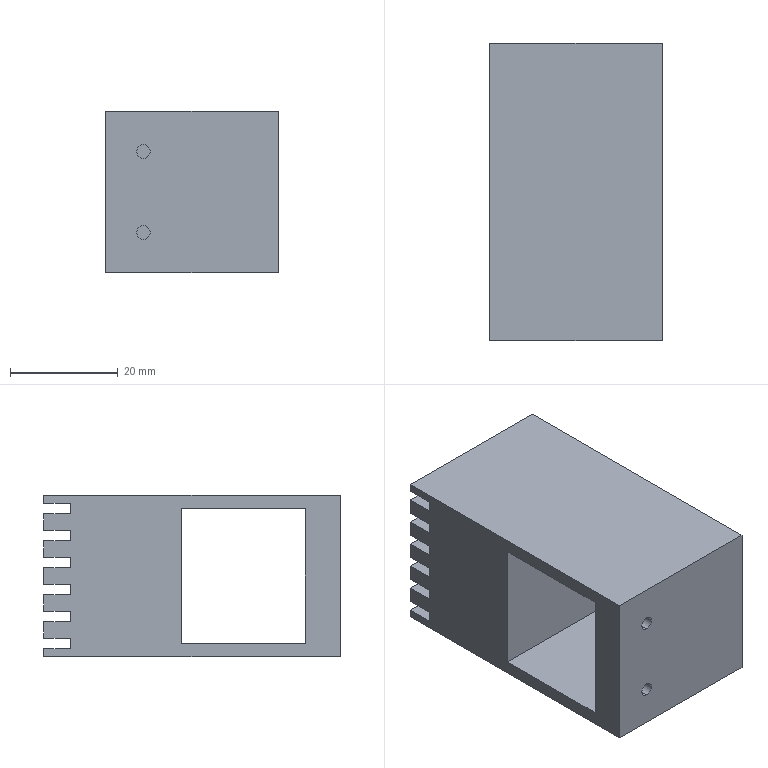Part | SolidWorks | features ICE 2, Extrusion 1, HoleWzd 1, LPattern 1 | 1 solid | 38 faces | box 32 x 55 x 30 mm | volume 32416 mm3 | plane 34 | cylinder 4 | commonest cylinder face diameters 2.5 x4
STEP:
#1=CARTESIAN_POINT('',(-9.,6.5,-8.75));
#2=VERTEX_POINT('',#1);
#3=CARTESIAN_POINT('',(-9.,6.5,-6.25));
#4=VERTEX_POINT('',#3);
#5=CARTESIAN_POINT('',(-9.,6.5,-7.5));
#6=DIRECTION('',(0.,1.,0.));
#7=DIRECTION('',(0.,0.,-1.));
#8=AXIS2_PLACEMENT_3D('',#5,#6,#7);
#9=CIRCLE('',#8,1.25);
#10=EDGE_CURVE('',#2,#4,#9,.T.);
#11=ORIENTED_EDGE('',*,*,#10,.T.);
#12=CARTESIAN_POINT('',(-9.,0.,-6.25));
#13=VERTEX_POINT('',#12);
#14=CARTESIAN_POINT('',(-9.,0.,-6.25));
#15=DIRECTION('',(0.,-1.,0.));
#16=VECTOR('',#15,1000.);
#17=LINE('',#14,#16);
#18=EDGE_CURVE('',#4,#13,#17,.T.);
#19=ORIENTED_EDGE('',*,*,#18,.T.);
#20=CARTESIAN_POINT('',(-9.,0.,-8.75));
#21=VERTEX_POINT('',#20);
#22=CARTESIAN_POINT('',(-9.,0.,-7.5));
#23=DIRECTION('',(0.,-1.,0.));
#24=DIRECTION('',(0.,0.,-1.));
#25=AXIS2_PLACEMENT_3D('',#22,#23,#24);
#26=CIRCLE('',#25,1.25);
#27=EDGE_CURVE('',#13,#21,#26,.T.);
#28=ORIENTED_EDGE('',*,*,#27,.T.);
#29=CARTESIAN_POINT('',(-9.,0.,-8.75));
#30=DIRECTION('',(0.,-1.,0.));
#31=VECTOR('',#30,1000.);
#32=LINE('',#29,#31);
#33=EDGE_CURVE('',#2,#21,#32,.T.);
#34=ORIENTED_EDGE('',*,*,#33,.F.);
#35=EDGE_LOOP('',(#11,#19,#28,#34));
#36=FACE_OUTER_BOUND('',#35,.T.);
#37=CARTESIAN_POINT('',(-9.,0.,-7.5));
#38=DIRECTION('',(0.,-1.,0.));
#39=DIRECTION('',(0.,0.,-1.));
#40=AXIS2_PLACEMENT_3D('',#37,#38,#39);
#41=CYLINDRICAL_SURFACE('',#40,1.25);
#42=ADVANCED_FACE('',(#36),#41,.F.);
#43=CARTESIAN_POINT('',(-9.,6.5,6.25));
#44=VERTEX_POINT('',#43);
#45=CARTESIAN_POINT('',(-9.,6.5,8.75));
#46=VERTEX_POINT('',#45);
#47=CARTESIAN_POINT('',(-9.,6.5,7.5));
#48=DIRECTION('',(0.,1.,0.));
#49=DIRECTION('',(0.,0.,-1.));
#50=AXIS2_PLACEMENT_3D('',#47,#48,#49);
#51=CIRCLE('',#50,1.25);
#52=EDGE_CURVE('',#44,#46,#51,.T.);
#53=ORIENTED_EDGE('',*,*,#52,.T.);
#54=CARTESIAN_POINT('',(-9.,0.,8.75));
#55=VERTEX_POINT('',#54);
#56=CARTESIAN_POINT('',(-9.,0.,8.75));
#57=DIRECTION('',(0.,-1.,0.));
#58=VECTOR('',#57,1000.);
#59=LINE('',#56,#58);
#60=EDGE_CURVE('',#46,#55,#59,.T.);
#61=ORIENTED_EDGE('',*,*,#60,.T.);
#62=CARTESIAN_POINT('',(-9.,0.,6.25));
#63=VERTEX_POINT('',#62);
#64=CARTESIAN_POINT('',(-9.,0.,7.5));
#65=DIRECTION('',(0.,-1.,0.));
#66=DIRECTION('',(0.,0.,-1.));
#67=AXIS2_PLACEMENT_3D('',#64,#65,#66);
#68=CIRCLE('',#67,1.25);
#69=EDGE_CURVE('',#55,#63,#68,.T.);
#70=ORIENTED_EDGE('',*,*,#69,.T.);
#71=CARTESIAN_POINT('',(-9.,0.,6.25));
#72=DIRECTION('',(0.,-1.,0.));
#73=VECTOR('',#72,1000.);
#74=LINE('',#71,#73);
#75=EDGE_CURVE('',#44,#63,#74,.T.);
#76=ORIENTED_EDGE('',*,*,#75,.F.);
#77=EDGE_LOOP('',(#53,#61,#70,#76));
#78=FACE_OUTER_BOUND('',#77,.T.);
#79=CARTESIAN_POINT('',(-9.,0.,7.5));
#80=DIRECTION('',(0.,-1.,0.));
#81=DIRECTION('',(0.,0.,-1.));
#82=AXIS2_PLACEMENT_3D('',#79,#80,#81);
#83=CYLINDRICAL_SURFACE('',#82,1.25);
#84=ADVANCED_FACE('',(#78),#83,.F.);
#85=CARTESIAN_POINT('',(-16.,55.,8.5));
#86=VERTEX_POINT('',#85);
#87=CARTESIAN_POINT('',(16.,55.,8.5));
#88=VERTEX_POINT('',#87);
#89=CARTESIAN_POINT('',(-16.,55.,8.5));
#90=DIRECTION('',(1.,0.,0.));
#91=VECTOR('',#90,1000.);
#92=LINE('',#89,#91);
#93=EDGE_CURVE('',#86,#88,#92,.T.);
#94=ORIENTED_EDGE('',*,*,#93,.F.);
#95=CARTESIAN_POINT('',(-16.,55.,11.5));
#96=VERTEX_POINT('',#95);
#97=CARTESIAN_POINT('',(-16.,55.,-15.));
#98=DIRECTION('',(0.,0.,1.));
#99=VECTOR('',#98,1000.);
#100=LINE('',#97,#99);
#101=EDGE_CURVE('',#86,#96,#100,.T.);
#102=ORIENTED_EDGE('',*,*,#101,.T.);
#103=CARTESIAN_POINT('',(16.,55.,11.5));
#104=VERTEX_POINT('',#103);
#105=CARTESIAN_POINT('',(-16.,55.,11.5));
#106=DIRECTION('',(1.,0.,0.));
#107=VECTOR('',#106,1000.);
#108=LINE('',#105,#107);
#109=EDGE_CURVE('',#96,#104,#108,.T.);
#110=ORIENTED_EDGE('',*,*,#109,.T.);
#111=CARTESIAN_POINT('',(16.,55.,-15.));
#112=DIRECTION('',(0.,0.,-1.));
#113=VECTOR('',#112,1000.);
#114=LINE('',#111,#113);
#115=EDGE_CURVE('',#104,#88,#114,.T.);
#116=ORIENTED_EDGE('',*,*,#115,.T.);
#117=EDGE_LOOP('',(#94,#102,#110,#116));
#118=FACE_OUTER_BOUND('',#117,.T.);
#119=CARTESIAN_POINT('',(0.,55.,0.));
#120=DIRECTION('',(0.,1.,0.));
#121=DIRECTION('',(0.,0.,1.));
#122=AXIS2_PLACEMENT_3D('',#119,#120,#121);
#123=PLANE('',#122);
#124=ADVANCED_FACE('',(#118),#123,.T.);
#125=CARTESIAN_POINT('',(-16.,55.,6.5));
#126=VERTEX_POINT('',#125);
#127=CARTESIAN_POINT('',(16.,55.,6.5));
#128=VERTEX_POINT('',#127);
#129=CARTESIAN_POINT('',(-16.,55.,6.5));
#130=DIRECTION('',(1.,0.,0.));
#131=VECTOR('',#130,1000.);
#132=LINE('',#129,#131);
#133=EDGE_CURVE('',#126,#128,#132,.T.);
#134=ORIENTED_EDGE('',*,*,#133,.T.);
#135=CARTESIAN_POINT('',(16.,55.,3.5));
#136=VERTEX_POINT('',#135);
#137=CARTESIAN_POINT('',(16.,55.,-15.));
#138=DIRECTION('',(0.,0.,-1.));
#139=VECTOR('',#138,1000.);
#140=LINE('',#137,#139);
#141=EDGE_CURVE('',#128,#136,#140,.T.);
#142=ORIENTED_EDGE('',*,*,#141,.T.);
#143=CARTESIAN_POINT('',(-16.,55.,3.5));
#144=VERTEX_POINT('',#143);
#145=CARTESIAN_POINT('',(-16.,55.,3.5));
#146=DIRECTION('',(1.,0.,0.));
#147=VECTOR('',#146,1000.);
#148=LINE('',#145,#147);
#149=EDGE_CURVE('',#144,#136,#148,.T.);
#150=ORIENTED_EDGE('',*,*,#149,.F.);
#151=CARTESIAN_POINT('',(-16.,55.,-15.));
#152=DIRECTION('',(0.,0.,1.));
#153=VECTOR('',#152,1000.);
#154=LINE('',#151,#153);
#155=EDGE_CURVE('',#144,#126,#154,.T.);
#156=ORIENTED_EDGE('',*,*,#155,.T.);
#157=EDGE_LOOP('',(#134,#142,#150,#156));
#158=FACE_OUTER_BOUND('',#157,.T.);
#159=CARTESIAN_POINT('',(0.,55.,0.));
#160=DIRECTION('',(0.,1.,0.));
#161=DIRECTION('',(0.,0.,1.));
#162=AXIS2_PLACEMENT_3D('',#159,#160,#161);
#163=PLANE('',#162);
#164=ADVANCED_FACE('',(#158),#163,.T.);
#165=CARTESIAN_POINT('',(-16.,55.,1.5));
#166=VERTEX_POINT('',#165);
#167=CARTESIAN_POINT('',(16.,55.,1.5));
#168=VERTEX_POINT('',#167);
#169=CARTESIAN_POINT('',(-16.,55.,1.5));
#170=DIRECTION('',(1.,0.,0.));
#171=VECTOR('',#170,1000.);
#172=LINE('',#169,#171);
#173=EDGE_CURVE('',#166,#168,#172,.T.);
#174=ORIENTED_EDGE('',*,*,#173,.T.);
#175=CARTESIAN_POINT('',(16.,55.,-1.5));
#176=VERTEX_POINT('',#175);
#177=CARTESIAN_POINT('',(16.,55.,-15.));
#178=DIRECTION('',(0.,0.,-1.));
#179=VECTOR('',#178,1000.);
#180=LINE('',#177,#179);
#181=EDGE_CURVE('',#168,#176,#180,.T.);
#182=ORIENTED_EDGE('',*,*,#181,.T.);
#183=CARTESIAN_POINT('',(-16.,55.,-1.5));
#184=VERTEX_POINT('',#183);
#185=CARTESIAN_POINT('',(-16.,55.,-1.5));
#186=DIRECTION('',(1.,0.,0.));
#187=VECTOR('',#186,1000.);
#188=LINE('',#185,#187);
#189=EDGE_CURVE('',#184,#176,#188,.T.);
#190=ORIENTED_EDGE('',*,*,#189,.F.);
#191=CARTESIAN_POINT('',(-16.,55.,-15.));
#192=DIRECTION('',(0.,0.,1.));
#193=VECTOR('',#192,1000.);
#194=LINE('',#191,#193);
#195=EDGE_CURVE('',#184,#166,#194,.T.);
#196=ORIENTED_EDGE('',*,*,#195,.T.);
#197=EDGE_LOOP('',(#174,#182,#190,#196));
#198=FACE_OUTER_BOUND('',#197,.T.);
#199=CARTESIAN_POINT('',(0.,55.,0.));
#200=DIRECTION('',(0.,1.,0.));
#201=DIRECTION('',(0.,0.,1.));
#202=AXIS2_PLACEMENT_3D('',#199,#200,#201);
#203=PLANE('',#202);
#204=ADVANCED_FACE('',(#198),#203,.T.);
#205=CARTESIAN_POINT('',(-16.,55.,-3.5));
#206=VERTEX_POINT('',#205);
#207=CARTESIAN_POINT('',(16.,55.,-3.5));
#208=VERTEX_POINT('',#207);
#209=CARTESIAN_POINT('',(-16.,55.,-3.5));
#210=DIRECTION('',(1.,0.,0.));
#211=VECTOR('',#210,1000.);
#212=LINE('',#209,#211);
#213=EDGE_CURVE('',#206,#208,#212,.T.);
#214=ORIENTED_EDGE('',*,*,#213,.T.);
#215=CARTESIAN_POINT('',(16.,55.,-6.5));
#216=VERTEX_POINT('',#215);
#217=CARTESIAN_POINT('',(16.,55.,-15.));
#218=DIRECTION('',(0.,0.,-1.));
#219=VECTOR('',#218,1000.);
#220=LINE('',#217,#219);
#221=EDGE_CURVE('',#208,#216,#220,.T.);
#222=ORIENTED_EDGE('',*,*,#221,.T.);
#223=CARTESIAN_POINT('',(-16.,55.,-6.5));
#224=VERTEX_POINT('',#223);
#225=CARTESIAN_POINT('',(-16.,55.,-6.5));
#226=DIRECTION('',(1.,0.,0.));
#227=VECTOR('',#226,1000.);
#228=LINE('',#225,#227);
#229=EDGE_CURVE('',#224,#216,#228,.T.);
#230=ORIENTED_EDGE('',*,*,#229,.F.);
#231=CARTESIAN_POINT('',(-16.,55.,-15.));
#232=DIRECTION('',(0.,0.,1.));
#233=VECTOR('',#232,1000.);
#234=LINE('',#231,#233);
#235=EDGE_CURVE('',#224,#206,#234,.T.);
#236=ORIENTED_EDGE('',*,*,#235,.T.);
#237=EDGE_LOOP('',(#214,#222,#230,#236));
#238=FACE_OUTER_BOUND('',#237,.T.);
#239=CARTESIAN_POINT('',(0.,55.,0.));
#240=DIRECTION('',(0.,1.,0.));
#241=DIRECTION('',(0.,0.,1.));
#242=AXIS2_PLACEMENT_3D('',#239,#240,#241);
#243=PLANE('',#242);
#244=ADVANCED_FACE('',(#238),#243,.T.);
#245=CARTESIAN_POINT('',(-16.,55.,-8.5));
#246=VERTEX_POINT('',#245);
#247=CARTESIAN_POINT('',(16.,55.,-8.5));
#248=VERTEX_POINT('',#247);
#249=CARTESIAN_POINT('',(-16.,55.,-8.5));
#250=DIRECTION('',(1.,0.,0.));
#251=VECTOR('',#250,1000.);
#252=LINE('',#249,#251);
#253=EDGE_CURVE('',#246,#248,#252,.T.);
#254=ORIENTED_EDGE('',*,*,#253,.T.);
#255=CARTESIAN_POINT('',(16.,55.,-11.5));
#256=VERTEX_POINT('',#255);
#257=CARTESIAN_POINT('',(16.,55.,-15.));
#258=DIRECTION('',(0.,0.,-1.));
#259=VECTOR('',#258,1000.);
#260=LINE('',#257,#259);
#261=EDGE_CURVE('',#248,#256,#260,.T.);
#262=ORIENTED_EDGE('',*,*,#261,.T.);
#263=CARTESIAN_POINT('',(-16.,55.,-11.5));
#264=VERTEX_POINT('',#263);
#265=CARTESIAN_POINT('',(-16.,55.,-11.5));
#266=DIRECTION('',(1.,0.,0.));
#267=VECTOR('',#266,1000.);
#268=LINE('',#265,#267);
#269=EDGE_CURVE('',#264,#256,#268,.T.);
#270=ORIENTED_EDGE('',*,*,#269,.F.);
#271=CARTESIAN_POINT('',(-16.,55.,-15.));
#272=DIRECTION('',(0.,0.,1.));
#273=VECTOR('',#272,1000.);
#274=LINE('',#271,#273);
#275=EDGE_CURVE('',#264,#246,#274,.T.);
#276=ORIENTED_EDGE('',*,*,#275,.T.);
#277=EDGE_LOOP('',(#254,#262,#270,#276));
#278=FACE_OUTER_BOUND('',#277,.T.);
#279=CARTESIAN_POINT('',(0.,55.,0.));
#280=DIRECTION('',(0.,1.,0.));
#281=DIRECTION('',(0.,0.,1.));
#282=AXIS2_PLACEMENT_3D('',#279,#280,#281);
#283=PLANE('',#282);
#284=ADVANCED_FACE('',(#278),#283,.T.);
#285=CARTESIAN_POINT('',(-16.,55.,13.5));
#286=VERTEX_POINT('',#285);
#287=CARTESIAN_POINT('',(16.,55.,13.5));
#288=VERTEX_POINT('',#287);
#289=CARTESIAN_POINT('',(-16.,55.,13.5));
#290=DIRECTION('',(1.,0.,0.));
#291=VECTOR('',#290,1000.);
#292=LINE('',#289,#291);
#293=EDGE_CURVE('',#286,#288,#292,.T.);
#294=ORIENTED_EDGE('',*,*,#293,.F.);
#295=CARTESIAN_POINT('',(-16.,55.,15.));
#296=VERTEX_POINT('',#295);
#297=CARTESIAN_POINT('',(-16.,55.,-15.));
#298=DIRECTION('',(0.,0.,1.));
#299=VECTOR('',#298,1000.);
#300=LINE('',#297,#299);
#301=EDGE_CURVE('',#286,#296,#300,.T.);
#302=ORIENTED_EDGE('',*,*,#301,.T.);
#303=CARTESIAN_POINT('',(16.,55.,15.));
#304=VERTEX_POINT('',#303);
#305=CARTESIAN_POINT('',(-16.,55.,15.));
#306=DIRECTION('',(1.,0.,0.));
#307=VECTOR('',#306,1000.);
#308=LINE('',#305,#307);
#309=EDGE_CURVE('',#296,#304,#308,.T.);
#310=ORIENTED_EDGE('',*,*,#309,.T.);
#311=CARTESIAN_POINT('',(16.,55.,-15.));
#312=DIRECTION('',(0.,0.,-1.));
#313=VECTOR('',#312,1000.);
#314=LINE('',#311,#313);
#315=EDGE_CURVE('',#304,#288,#314,.T.);
#316=ORIENTED_EDGE('',*,*,#315,.T.);
#317=EDGE_LOOP('',(#294,#302,#310,#316));
#318=FACE_OUTER_BOUND('',#317,.T.);
#319=CARTESIAN_POINT('',(0.,55.,0.));
#320=DIRECTION('',(0.,1.,0.));
#321=DIRECTION('',(0.,0.,1.));
#322=AXIS2_PLACEMENT_3D('',#319,#320,#321);
#323=PLANE('',#322);
#324=ADVANCED_FACE('',(#318),#323,.T.);
#325=CARTESIAN_POINT('',(16.,6.5,12.5));
#326=VERTEX_POINT('',#325);
#327=CARTESIAN_POINT('',(16.,6.5,-12.5));
#328=VERTEX_POINT('',#327);
#329=CARTESIAN_POINT('',(16.,6.5,12.5));
#330=DIRECTION('',(0.,0.,-1.));
#331=VECTOR('',#330,1000.);
#332=LINE('',#329,#331);
#333=EDGE_CURVE('',#326,#328,#332,.T.);
#334=ORIENTED_EDGE('',*,*,#333,.F.);
#335=CARTESIAN_POINT('',(16.,29.5,12.5));
#336=VERTEX_POINT('',#335);
#337=CARTESIAN_POINT('',(16.,6.5,12.5));
#338=DIRECTION('',(0.,-1.,0.));
#339=VECTOR('',#338,1000.);
#340=LINE('',#337,#339);
#341=EDGE_CURVE('',#336,#326,#340,.T.);
#342=ORIENTED_EDGE('',*,*,#341,.F.);
#343=CARTESIAN_POINT('',(16.,29.5,-12.5));
#344=VERTEX_POINT('',#343);
#345=CARTESIAN_POINT('',(16.,29.5,12.5));
#346=DIRECTION('',(0.,0.,1.));
#347=VECTOR('',#346,1000.);
#348=LINE('',#345,#347);
#349=EDGE_CURVE('',#344,#336,#348,.T.);
#350=ORIENTED_EDGE('',*,*,#349,.F.);
#351=CARTESIAN_POINT('',(16.,6.5,-12.5));
#352=DIRECTION('',(0.,1.,0.));
#353=VECTOR('',#352,1000.);
#354=LINE('',#351,#353);
#355=EDGE_CURVE('',#328,#344,#354,.T.);
#356=ORIENTED_EDGE('',*,*,#355,.F.);
#357=EDGE_LOOP('',(#334,#342,#350,#356));
#358=FACE_BOUND('',#357,.T.);
#359=CARTESIAN_POINT('',(16.,50.,8.5));
#360=VERTEX_POINT('',#359);
#361=CARTESIAN_POINT('',(16.,50.,6.5));
#362=VERTEX_POINT('',#361);
#363=CARTESIAN_POINT('',(16.,50.,8.5));
#364=DIRECTION('',(0.,0.,-1.));
#365=VECTOR('',#364,1000.);
#366=LINE('',#363,#365);
#367=EDGE_CURVE('',#360,#362,#366,.T.);
#368=ORIENTED_EDGE('',*,*,#367,.F.);
#369=CARTESIAN_POINT('',(16.,55.,8.5));
#370=DIRECTION('',(0.,-1.,0.));
#371=VECTOR('',#370,1000.);
#372=LINE('',#369,#371);
#373=EDGE_CURVE('',#88,#360,#372,.T.);
#374=ORIENTED_EDGE('',*,*,#373,.F.);
#375=ORIENTED_EDGE('',*,*,#115,.F.);
#376=CARTESIAN_POINT('',(16.,50.,11.5));
#377=VERTEX_POINT('',#376);
#378=CARTESIAN_POINT('',(16.,55.,11.5));
#379=DIRECTION('',(0.,1.,0.));
#380=VECTOR('',#379,1000.);
#381=LINE('',#378,#380);
#382=EDGE_CURVE('',#377,#104,#381,.T.);
#383=ORIENTED_EDGE('',*,*,#382,.F.);
#384=CARTESIAN_POINT('',(16.,50.,13.5));
#385=VERTEX_POINT('',#384);
#386=CARTESIAN_POINT('',(16.,50.,13.5));
#387=DIRECTION('',(0.,0.,-1.));
#388=VECTOR('',#387,1000.);
#389=LINE('',#386,#388);
#390=EDGE_CURVE('',#385,#377,#389,.T.);
#391=ORIENTED_EDGE('',*,*,#390,.F.);
#392=CARTESIAN_POINT('',(16.,55.,13.5));
#393=DIRECTION('',(0.,-1.,0.));
#394=VECTOR('',#393,1000.);
#395=LINE('',#392,#394);
#396=EDGE_CURVE('',#288,#385,#395,.T.);
#397=ORIENTED_EDGE('',*,*,#396,.F.);
#398=ORIENTED_EDGE('',*,*,#315,.F.);
#399=CARTESIAN_POINT('',(16.,0.,15.));
#400=VERTEX_POINT('',#399);
#401=CARTESIAN_POINT('',(16.,55.,15.));
#402=DIRECTION('',(0.,-1.,0.));
#403=VECTOR('',#402,1000.);
#404=LINE('',#401,#403);
#405=EDGE_CURVE('',#304,#400,#404,.T.);
#406=ORIENTED_EDGE('',*,*,#405,.T.);
#407=CARTESIAN_POINT('',(16.,0.,-15.));
#408=VERTEX_POINT('',#407);
#409=CARTESIAN_POINT('',(16.,0.,-15.));
#410=DIRECTION('',(0.,0.,-1.));
#411=VECTOR('',#410,1000.);
#412=LINE('',#409,#411);
#413=EDGE_CURVE('',#400,#408,#412,.T.);
#414=ORIENTED_EDGE('',*,*,#413,.T.);
#415=CARTESIAN_POINT('',(16.,55.,-15.));
#416=VERTEX_POINT('',#415);
#417=CARTESIAN_POINT('',(16.,55.,-15.));
#418=DIRECTION('',(0.,-1.,0.));
#419=VECTOR('',#418,1000.);
#420=LINE('',#417,#419);
#421=EDGE_CURVE('',#416,#408,#420,.T.);
#422=ORIENTED_EDGE('',*,*,#421,.F.);
#423=CARTESIAN_POINT('',(16.,55.,-13.5));
#424=VERTEX_POINT('',#423);
#425=CARTESIAN_POINT('',(16.,55.,-15.));
#426=DIRECTION('',(0.,0.,-1.));
#427=VECTOR('',#426,1000.);
#428=LINE('',#425,#427);
#429=EDGE_CURVE('',#424,#416,#428,.T.);
#430=ORIENTED_EDGE('',*,*,#429,.F.);
#431=CARTESIAN_POINT('',(16.,50.,-13.5));
#432=VERTEX_POINT('',#431);
#433=CARTESIAN_POINT('',(16.,55.,-13.5));
#434=DIRECTION('',(0.,1.,0.));
#435=VECTOR('',#434,1000.);
#436=LINE('',#433,#435);
#437=EDGE_CURVE('',#432,#424,#436,.T.);
#438=ORIENTED_EDGE('',*,*,#437,.F.);
#439=CARTESIAN_POINT('',(16.,50.,-11.5));
#440=VERTEX_POINT('',#439);
#441=CARTESIAN_POINT('',(16.,50.,-11.5));
#442=DIRECTION('',(0.,0.,-1.));
#443=VECTOR('',#442,1000.);
#444=LINE('',#441,#443);
#445=EDGE_CURVE('',#440,#432,#444,.T.);
#446=ORIENTED_EDGE('',*,*,#445,.F.);
#447=CARTESIAN_POINT('',(16.,55.,-11.5));
#448=DIRECTION('',(0.,-1.,0.));
#449=VECTOR('',#448,1000.);
#450=LINE('',#447,#449);
#451=EDGE_CURVE('',#256,#440,#450,.T.);
#452=ORIENTED_EDGE('',*,*,#451,.F.);
#453=ORIENTED_EDGE('',*,*,#261,.F.);
#454=CARTESIAN_POINT('',(16.,50.,-8.5));
#455=VERTEX_POINT('',#454);
#456=CARTESIAN_POINT('',(16.,55.,-8.5));
#457=DIRECTION('',(0.,1.,0.));
#458=VECTOR('',#457,1000.);
#459=LINE('',#456,#458);
#460=EDGE_CURVE('',#455,#248,#459,.T.);
#461=ORIENTED_EDGE('',*,*,#460,.F.);
#462=CARTESIAN_POINT('',(16.,50.,-6.5));
#463=VERTEX_POINT('',#462);
#464=CARTESIAN_POINT('',(16.,50.,-6.5));
#465=DIRECTION('',(0.,0.,-1.));
#466=VECTOR('',#465,1000.);
#467=LINE('',#464,#466);
#468=EDGE_CURVE('',#463,#455,#467,.T.);
#469=ORIENTED_EDGE('',*,*,#468,.F.);
#470=CARTESIAN_POINT('',(16.,55.,-6.5));
#471=DIRECTION('',(0.,-1.,0.));
#472=VECTOR('',#471,1000.);
#473=LINE('',#470,#472);
#474=EDGE_CURVE('',#216,#463,#473,.T.);
#475=ORIENTED_EDGE('',*,*,#474,.F.);
#476=ORIENTED_EDGE('',*,*,#221,.F.);
#477=CARTESIAN_POINT('',(16.,50.,-3.5));
#478=VERTEX_POINT('',#477);
#479=CARTESIAN_POINT('',(16.,55.,-3.5));
#480=DIRECTION('',(0.,1.,0.));
#481=VECTOR('',#480,1000.);
#482=LINE('',#479,#481);
#483=EDGE_CURVE('',#478,#208,#482,.T.);
#484=ORIENTED_EDGE('',*,*,#483,.F.);
#485=CARTESIAN_POINT('',(16.,50.,-1.5));
#486=VERTEX_POINT('',#485);
#487=CARTESIAN_POINT('',(16.,50.,-1.5));
#488=DIRECTION('',(0.,0.,-1.));
#489=VECTOR('',#488,1000.);
#490=LINE('',#487,#489);
#491=EDGE_CURVE('',#486,#478,#490,.T.);
#492=ORIENTED_EDGE('',*,*,#491,.F.);
#493=CARTESIAN_POINT('',(16.,55.,-1.5));
#494=DIRECTION('',(0.,-1.,0.));
#495=VECTOR('',#494,1000.);
#496=LINE('',#493,#495);
#497=EDGE_CURVE('',#176,#486,#496,.T.);
#498=ORIENTED_EDGE('',*,*,#497,.F.);
#499=ORIENTED_EDGE('',*,*,#181,.F.);
#500=CARTESIAN_POINT('',(16.,50.,1.5));
#501=VERTEX_POINT('',#500);
#502=CARTESIAN_POINT('',(16.,55.,1.5));
#503=DIRECTION('',(0.,1.,0.));
#504=VECTOR('',#503,1000.);
#505=LINE('',#502,#504);
#506=EDGE_CURVE('',#501,#168,#505,.T.);
#507=ORIENTED_EDGE('',*,*,#506,.F.);
#508=CARTESIAN_POINT('',(16.,50.,3.5));
#509=VERTEX_POINT('',#508);
#510=CARTESIAN_POINT('',(16.,50.,3.5));
#511=DIRECTION('',(0.,0.,-1.));
#512=VECTOR('',#511,1000.);
#513=LINE('',#510,#512);
#514=EDGE_CURVE('',#509,#501,#513,.T.);
#515=ORIENTED_EDGE('',*,*,#514,.F.);
#516=CARTESIAN_POINT('',(16.,55.,3.5));
#517=DIRECTION('',(0.,-1.,0.));
#518=VECTOR('',#517,1000.);
#519=LINE('',#516,#518);
#520=EDGE_CURVE('',#136,#509,#519,.T.);
#521=ORIENTED_EDGE('',*,*,#520,.F.);
#522=ORIENTED_EDGE('',*,*,#141,.F.);
#523=CARTESIAN_POINT('',(16.,55.,6.5));
#524=DIRECTION('',(0.,1.,0.));
#525=VECTOR('',#524,1000.);
#526=LINE('',#523,#525);
#527=EDGE_CURVE('',#362,#128,#526,.T.);
#528=ORIENTED_EDGE('',*,*,#527,.F.);
#529=EDGE_LOOP('',(#368,#374,#375,#383,#391,#397,#398,#406,#414,#422,#430,#438,#446,#452,#453,#461,#469,#475,#476,#484,#492,#498,#499,#507,#515,#521,#522,#528));
#530=FACE_OUTER_BOUND('',#529,.T.);
#531=CARTESIAN_POINT('',(16.,55.,-15.));
#532=DIRECTION('',(-1.,0.,0.));
#533=DIRECTION('',(0.,0.,1.));
#534=AXIS2_PLACEMENT_3D('',#531,#532,#533);
#535=PLANE('',#534);
#536=ADVANCED_FACE('',(#358,#530),#535,.F.);
#537=CARTESIAN_POINT('',(-16.,0.,-15.));
#538=VERTEX_POINT('',#537);
#539=CARTESIAN_POINT('',(-16.,0.,-15.));
#540=DIRECTION('',(-1.,0.,0.));
#541=VECTOR('',#540,1000.);
#542=LINE('',#539,#541);
#543=EDGE_CURVE('',#408,#538,#542,.T.);
#544=ORIENTED_EDGE('',*,*,#543,.T.);
#545=CARTESIAN_POINT('',(-16.,55.,-15.));
#546=VERTEX_POINT('',#545);
#547=CARTESIAN_POINT('',(-16.,55.,-15.));
#548=DIRECTION('',(0.,-1.,0.));
#549=VECTOR('',#548,1000.);
#550=LINE('',#547,#549);
#551=EDGE_CURVE('',#546,#538,#550,.T.);
#552=ORIENTED_EDGE('',*,*,#551,.F.);
#553=CARTESIAN_POINT('',(-16.,55.,-15.));
#554=DIRECTION('',(-1.,0.,0.));
#555=VECTOR('',#554,1000.);
#556=LINE('',#553,#555);
#557=EDGE_CURVE('',#416,#546,#556,.T.);
#558=ORIENTED_EDGE('',*,*,#557,.F.);
#559=ORIENTED_EDGE('',*,*,#421,.T.);
#560=EDGE_LOOP('',(#544,#552,#558,#559));
#561=FACE_OUTER_BOUND('',#560,.T.);
#562=CARTESIAN_POINT('',(-16.,55.,-15.));
#563=DIRECTION('',(0.,0.,1.));
#564=DIRECTION('',(1.,0.,0.));
#565=AXIS2_PLACEMENT_3D('',#562,#563,#564);
#566=PLANE('',#565);
#567=ADVANCED_FACE('',(#561),#566,.F.);
#568=ORIENTED_EDGE('',*,*,#101,.F.);
#569=CARTESIAN_POINT('',(-16.,50.,8.5));
#570=VERTEX_POINT('',#569);
#571=CARTESIAN_POINT('',(-16.,55.,8.5));
#572=DIRECTION('',(0.,-1.,0.));
#573=VECTOR('',#572,1000.);
#574=LINE('',#571,#573);
#575=EDGE_CURVE('',#86,#570,#574,.T.);
#576=ORIENTED_EDGE('',*,*,#575,.T.);
#577=CARTESIAN_POINT('',(-16.,50.,6.5));
#578=VERTEX_POINT('',#577);
#579=CARTESIAN_POINT('',(-16.,50.,8.5));
#580=DIRECTION('',(0.,0.,-1.));
#581=VECTOR('',#580,1000.);
#582=LINE('',#579,#581);
#583=EDGE_CURVE('',#570,#578,#582,.T.);
#584=ORIENTED_EDGE('',*,*,#583,.T.);
#585=CARTESIAN_POINT('',(-16.,55.,6.5));
#586=DIRECTION('',(0.,1.,0.));
#587=VECTOR('',#586,1000.);
#588=LINE('',#585,#587);
#589=EDGE_CURVE('',#578,#126,#588,.T.);
#590=ORIENTED_EDGE('',*,*,#589,.T.);
#591=ORIENTED_EDGE('',*,*,#155,.F.);
#592=CARTESIAN_POINT('',(-16.,50.,3.5));
#593=VERTEX_POINT('',#592);
#594=CARTESIAN_POINT('',(-16.,55.,3.5));
#595=DIRECTION('',(0.,-1.,0.));
#596=VECTOR('',#595,1000.);
#597=LINE('',#594,#596);
#598=EDGE_CURVE('',#144,#593,#597,.T.);
#599=ORIENTED_EDGE('',*,*,#598,.T.);
#600=CARTESIAN_POINT('',(-16.,50.,1.5));
#601=VERTEX_POINT('',#600);
#602=CARTESIAN_POINT('',(-16.,50.,3.5));
#603=DIRECTION('',(0.,0.,-1.));
#604=VECTOR('',#603,1000.);
#605=LINE('',#602,#604);
#606=EDGE_CURVE('',#593,#601,#605,.T.);
#607=ORIENTED_EDGE('',*,*,#606,.T.);
#608=CARTESIAN_POINT('',(-16.,55.,1.5));
#609=DIRECTION('',(0.,1.,0.));
#610=VECTOR('',#609,1000.);
#611=LINE('',#608,#610);
#612=EDGE_CURVE('',#601,#166,#611,.T.);
#613=ORIENTED_EDGE('',*,*,#612,.T.);
#614=ORIENTED_EDGE('',*,*,#195,.F.);
#615=CARTESIAN_POINT('',(-16.,50.,-1.5));
#616=VERTEX_POINT('',#615);
#617=CARTESIAN_POINT('',(-16.,55.,-1.5));
#618=DIRECTION('',(0.,-1.,0.));
#619=VECTOR('',#618,1000.);
#620=LINE('',#617,#619);
#621=EDGE_CURVE('',#184,#616,#620,.T.);
#622=ORIENTED_EDGE('',*,*,#621,.T.);
#623=CARTESIAN_POINT('',(-16.,50.,-3.5));
#624=VERTEX_POINT('',#623);
#625=CARTESIAN_POINT('',(-16.,50.,-1.5));
#626=DIRECTION('',(0.,0.,-1.));
#627=VECTOR('',#626,1000.);
#628=LINE('',#625,#627);
#629=EDGE_CURVE('',#616,#624,#628,.T.);
#630=ORIENTED_EDGE('',*,*,#629,.T.);
#631=CARTESIAN_POINT('',(-16.,55.,-3.5));
#632=DIRECTION('',(0.,1.,0.));
#633=VECTOR('',#632,1000.);
#634=LINE('',#631,#633);
#635=EDGE_CURVE('',#624,#206,#634,.T.);
#636=ORIENTED_EDGE('',*,*,#635,.T.);
#637=ORIENTED_EDGE('',*,*,#235,.F.);
#638=CARTESIAN_POINT('',(-16.,50.,-6.5));
#639=VERTEX_POINT('',#638);
#640=CARTESIAN_POINT('',(-16.,55.,-6.5));
#641=DIRECTION('',(0.,-1.,0.));
#642=VECTOR('',#641,1000.);
#643=LINE('',#640,#642);
#644=EDGE_CURVE('',#224,#639,#643,.T.);
#645=ORIENTED_EDGE('',*,*,#644,.T.);
#646=CARTESIAN_POINT('',(-16.,50.,-8.5));
#647=VERTEX_POINT('',#646);
#648=CARTESIAN_POINT('',(-16.,50.,-6.5));
#649=DIRECTION('',(0.,0.,-1.));
#650=VECTOR('',#649,1000.);
#651=LINE('',#648,#650);
#652=EDGE_CURVE('',#639,#647,#651,.T.);
#653=ORIENTED_EDGE('',*,*,#652,.T.);
#654=CARTESIAN_POINT('',(-16.,55.,-8.5));
#655=DIRECTION('',(0.,1.,0.));
#656=VECTOR('',#655,1000.);
#657=LINE('',#654,#656);
#658=EDGE_CURVE('',#647,#246,#657,.T.);
#659=ORIENTED_EDGE('',*,*,#658,.T.);
#660=ORIENTED_EDGE('',*,*,#275,.F.);
#661=CARTESIAN_POINT('',(-16.,50.,-11.5));
#662=VERTEX_POINT('',#661);
#663=CARTESIAN_POINT('',(-16.,55.,-11.5));
#664=DIRECTION('',(0.,-1.,0.));
#665=VECTOR('',#664,1000.);
#666=LINE('',#663,#665);
#667=EDGE_CURVE('',#264,#662,#666,.T.);
#668=ORIENTED_EDGE('',*,*,#667,.T.);
#669=CARTESIAN_POINT('',(-16.,50.,-13.5));
#670=VERTEX_POINT('',#669);
#671=CARTESIAN_POINT('',(-16.,50.,-11.5));
#672=DIRECTION('',(0.,0.,-1.));
#673=VECTOR('',#672,1000.);
#674=LINE('',#671,#673);
#675=EDGE_CURVE('',#662,#670,#674,.T.);
#676=ORIENTED_EDGE('',*,*,#675,.T.);
#677=CARTESIAN_POINT('',(-16.,55.,-13.5));
#678=VERTEX_POINT('',#677);
#679=CARTESIAN_POINT('',(-16.,55.,-13.5));
#680=DIRECTION('',(0.,1.,0.));
#681=VECTOR('',#680,1000.);
#682=LINE('',#679,#681);
#683=EDGE_CURVE('',#670,#678,#682,.T.);
#684=ORIENTED_EDGE('',*,*,#683,.T.);
#685=CARTESIAN_POINT('',(-16.,55.,-15.));
#686=DIRECTION('',(0.,0.,1.));
#687=VECTOR('',#686,1000.);
#688=LINE('',#685,#687);
#689=EDGE_CURVE('',#546,#678,#688,.T.);
#690=ORIENTED_EDGE('',*,*,#689,.F.);
#691=ORIENTED_EDGE('',*,*,#551,.T.);
#692=CARTESIAN_POINT('',(-16.,0.,15.));
#693=VERTEX_POINT('',#692);
#694=CARTESIAN_POINT('',(-16.,0.,-15.));
#695=DIRECTION('',(0.,0.,1.));
#696=VECTOR('',#695,1000.);
#697=LINE('',#694,#696);
#698=EDGE_CURVE('',#538,#693,#697,.T.);
#699=ORIENTED_EDGE('',*,*,#698,.T.);
#700=CARTESIAN_POINT('',(-16.,55.,15.));
#701=DIRECTION('',(0.,-1.,0.));
#702=VECTOR('',#701,1000.);
#703=LINE('',#700,#702);
#704=EDGE_CURVE('',#296,#693,#703,.T.);
#705=ORIENTED_EDGE('',*,*,#704,.F.);
#706=ORIENTED_EDGE('',*,*,#301,.F.);
#707=CARTESIAN_POINT('',(-16.,50.,13.5));
#708=VERTEX_POINT('',#707);
#709=CARTESIAN_POINT('',(-16.,55.,13.5));
#710=DIRECTION('',(0.,-1.,0.));
#711=VECTOR('',#710,1000.);
#712=LINE('',#709,#711);
#713=EDGE_CURVE('',#286,#708,#712,.T.);
#714=ORIENTED_EDGE('',*,*,#713,.T.);
#715=CARTESIAN_POINT('',(-16.,50.,11.5));
#716=VERTEX_POINT('',#715);
#717=CARTESIAN_POINT('',(-16.,50.,13.5));
#718=DIRECTION('',(0.,0.,-1.));
#719=VECTOR('',#718,1000.);
#720=LINE('',#717,#719);
#721=EDGE_CURVE('',#708,#716,#720,.T.);
#722=ORIENTED_EDGE('',*,*,#721,.T.);
#723=CARTESIAN_POINT('',(-16.,55.,11.5));
#724=DIRECTION('',(0.,1.,0.));
#725=VECTOR('',#724,1000.);
#726=LINE('',#723,#725);
#727=EDGE_CURVE('',#716,#96,#726,.T.);
#728=ORIENTED_EDGE('',*,*,#727,.T.);
#729=EDGE_LOOP('',(#568,#576,#584,#590,#591,#599,#607,#613,#614,#622,#630,#636,#637,#645,#653,#659,#660,#668,#676,#684,#690,#691,#699,#705,#706,#714,#722,#728));
#730=FACE_OUTER_BOUND('',#729,.T.);
#731=CARTESIAN_POINT('',(-16.,29.5,-12.5));
#732=VERTEX_POINT('',#731);
#733=CARTESIAN_POINT('',(-16.,29.5,12.5));
#734=VERTEX_POINT('',#733);
#735=CARTESIAN_POINT('',(-16.,29.5,-15.));
#736=DIRECTION('',(0.,0.,1.));
#737=VECTOR('',#736,1000.);
#738=LINE('',#735,#737);
#739=EDGE_CURVE('',#732,#734,#738,.T.);
#740=ORIENTED_EDGE('',*,*,#739,.T.);
#741=CARTESIAN_POINT('',(-16.,6.5,12.5));
#742=VERTEX_POINT('',#741);
#743=CARTESIAN_POINT('',(-16.,55.,12.5));
#744=DIRECTION('',(0.,-1.,0.));
#745=VECTOR('',#744,1000.);
#746=LINE('',#743,#745);
#747=EDGE_CURVE('',#734,#742,#746,.T.);
#748=ORIENTED_EDGE('',*,*,#747,.T.);
#749=CARTESIAN_POINT('',(-16.,6.5,-12.5));
#750=VERTEX_POINT('',#749);
#751=CARTESIAN_POINT('',(-16.,6.5,-15.));
#752=DIRECTION('',(0.,0.,-1.));
#753=VECTOR('',#752,1000.);
#754=LINE('',#751,#753);
#755=EDGE_CURVE('',#742,#750,#754,.T.);
#756=ORIENTED_EDGE('',*,*,#755,.T.);
#757=CARTESIAN_POINT('',(-16.,55.,-12.5));
#758=DIRECTION('',(0.,1.,0.));
#759=VECTOR('',#758,1000.);
#760=LINE('',#757,#759);
#761=EDGE_CURVE('',#750,#732,#760,.T.);
#762=ORIENTED_EDGE('',*,*,#761,.T.);
#763=EDGE_LOOP('',(#740,#748,#756,#762));
#764=FACE_BOUND('',#763,.T.);
#765=CARTESIAN_POINT('',(-16.,55.,-15.));
#766=DIRECTION('',(1.,0.,0.));
#767=DIRECTION('',(0.,0.,-1.));
#768=AXIS2_PLACEMENT_3D('',#765,#766,#767);
#769=PLANE('',#768);
#770=ADVANCED_FACE('',(#730,#764),#769,.F.);
#771=CARTESIAN_POINT('',(-16.,0.,15.));
#772=DIRECTION('',(1.,0.,0.));
#773=VECTOR('',#772,1000.);
#774=LINE('',#771,#773);
#775=EDGE_CURVE('',#693,#400,#774,.T.);
#776=ORIENTED_EDGE('',*,*,#775,.T.);
#777=ORIENTED_EDGE('',*,*,#405,.F.);
#778=ORIENTED_EDGE('',*,*,#309,.F.);
#779=ORIENTED_EDGE('',*,*,#704,.T.);
#780=EDGE_LOOP('',(#776,#777,#778,#779));
#781=FACE_OUTER_BOUND('',#780,.T.);
#782=CARTESIAN_POINT('',(-16.,55.,15.));
#783=DIRECTION('',(0.,0.,-1.));
#784=DIRECTION('',(-1.,0.,0.));
#785=AXIS2_PLACEMENT_3D('',#782,#783,#784);
#786=PLANE('',#785);
#787=ADVANCED_FACE('',(#781),#786,.F.);
#788=CARTESIAN_POINT('',(-16.,55.,-13.5));
#789=DIRECTION('',(1.,0.,0.));
#790=VECTOR('',#789,1000.);
#791=LINE('',#788,#790);
#792=EDGE_CURVE('',#678,#424,#791,.T.);
#793=ORIENTED_EDGE('',*,*,#792,.T.);
#794=ORIENTED_EDGE('',*,*,#429,.T.);
#795=ORIENTED_EDGE('',*,*,#557,.T.);
#796=ORIENTED_EDGE('',*,*,#689,.T.);
#797=EDGE_LOOP('',(#793,#794,#795,#796));
#798=FACE_OUTER_BOUND('',#797,.T.);
#799=CARTESIAN_POINT('',(0.,55.,0.));
#800=DIRECTION('',(0.,1.,0.));
#801=DIRECTION('',(0.,0.,1.));
#802=AXIS2_PLACEMENT_3D('',#799,#800,#801);
#803=PLANE('',#802);
#804=ADVANCED_FACE('',(#798),#803,.T.);
#805=CARTESIAN_POINT('',(-9.,0.,-7.5));
#806=DIRECTION('',(0.,-1.,0.));
#807=DIRECTION('',(0.,0.,-1.));
#808=AXIS2_PLACEMENT_3D('',#805,#806,#807);
#809=CIRCLE('',#808,1.25);
#810=EDGE_CURVE('',#21,#13,#809,.T.);
#811=ORIENTED_EDGE('',*,*,#810,.F.);
#812=ORIENTED_EDGE('',*,*,#27,.F.);
#813=EDGE_LOOP('',(#811,#812));
#814=FACE_BOUND('',#813,.T.);
#815=CARTESIAN_POINT('',(-9.,0.,7.5));
#816=DIRECTION('',(0.,-1.,0.));
#817=DIRECTION('',(0.,0.,-1.));
#818=AXIS2_PLACEMENT_3D('',#815,#816,#817);
#819=CIRCLE('',#818,1.25);
#820=EDGE_CURVE('',#63,#55,#819,.T.);
#821=ORIENTED_EDGE('',*,*,#820,.F.);
#822=ORIENTED_EDGE('',*,*,#69,.F.);
#823=EDGE_LOOP('',(#821,#822));
#824=FACE_BOUND('',#823,.T.);
#825=ORIENTED_EDGE('',*,*,#413,.F.);
#826=ORIENTED_EDGE('',*,*,#775,.F.);
#827=ORIENTED_EDGE('',*,*,#698,.F.);
#828=ORIENTED_EDGE('',*,*,#543,.F.);
#829=EDGE_LOOP('',(#825,#826,#827,#828));
#830=FACE_OUTER_BOUND('',#829,.T.);
#831=CARTESIAN_POINT('',(0.,0.,0.));
#832=DIRECTION('',(0.,1.,0.));
#833=DIRECTION('',(0.,0.,1.));
#834=AXIS2_PLACEMENT_3D('',#831,#832,#833);
#835=PLANE('',#834);
#836=ADVANCED_FACE('',(#814,#824,#830),#835,.F.);
#837=ORIENTED_EDGE('',*,*,#60,.F.);
#838=CARTESIAN_POINT('',(-9.,6.5,7.5));
#839=DIRECTION('',(0.,1.,0.));
#840=DIRECTION('',(0.,0.,-1.));
#841=AXIS2_PLACEMENT_3D('',#838,#839,#840);
#842=CIRCLE('',#841,1.25);
#843=EDGE_CURVE('',#46,#44,#842,.T.);
#844=ORIENTED_EDGE('',*,*,#843,.T.);
#845=ORIENTED_EDGE('',*,*,#75,.T.);
#846=ORIENTED_EDGE('',*,*,#820,.T.);
#847=EDGE_LOOP('',(#837,#844,#845,#846));
#848=FACE_OUTER_BOUND('',#847,.T.);
#849=CARTESIAN_POINT('',(-9.,0.,7.5));
#850=DIRECTION('',(0.,-1.,0.));
#851=DIRECTION('',(0.,0.,-1.));
#852=AXIS2_PLACEMENT_3D('',#849,#850,#851);
#853=CYLINDRICAL_SURFACE('',#852,1.25);
#854=ADVANCED_FACE('',(#848),#853,.F.);
#855=ORIENTED_EDGE('',*,*,#18,.F.);
#856=CARTESIAN_POINT('',(-9.,6.5,-7.5));
#857=DIRECTION('',(0.,1.,0.));
#858=DIRECTION('',(0.,0.,-1.));
#859=AXIS2_PLACEMENT_3D('',#856,#857,#858);
#860=CIRCLE('',#859,1.25);
#861=EDGE_CURVE('',#4,#2,#860,.T.);
#862=ORIENTED_EDGE('',*,*,#861,.T.);
#863=ORIENTED_EDGE('',*,*,#33,.T.);
#864=ORIENTED_EDGE('',*,*,#810,.T.);
#865=EDGE_LOOP('',(#855,#862,#863,#864));
#866=FACE_OUTER_BOUND('',#865,.T.);
#867=CARTESIAN_POINT('',(-9.,0.,-7.5));
#868=DIRECTION('',(0.,-1.,0.));
#869=DIRECTION('',(0.,0.,-1.));
#870=AXIS2_PLACEMENT_3D('',#867,#868,#869);
#871=CYLINDRICAL_SURFACE('',#870,1.25);
#872=ADVANCED_FACE('',(#866),#871,.F.);
#873=CARTESIAN_POINT('',(-44.,29.5,12.5));
#874=DIRECTION('',(1.,0.,0.));
#875=VECTOR('',#874,1000.);
#876=LINE('',#873,#875);
#877=EDGE_CURVE('',#734,#336,#876,.T.);
#878=ORIENTED_EDGE('',*,*,#877,.T.);
#879=ORIENTED_EDGE('',*,*,#341,.T.);
#880=CARTESIAN_POINT('',(-44.,6.5,12.5));
#881=DIRECTION('',(1.,0.,0.));
#882=VECTOR('',#881,1000.);
#883=LINE('',#880,#882);
#884=EDGE_CURVE('',#742,#326,#883,.T.);
#885=ORIENTED_EDGE('',*,*,#884,.F.);
#886=ORIENTED_EDGE('',*,*,#747,.F.);
#887=EDGE_LOOP('',(#878,#879,#885,#886));
#888=FACE_OUTER_BOUND('',#887,.T.);
#889=CARTESIAN_POINT('',(-44.,6.5,12.5));
#890=DIRECTION('',(0.,0.,1.));
#891=DIRECTION('',(1.,0.,0.));
#892=AXIS2_PLACEMENT_3D('',#889,#890,#891);
#893=PLANE('',#892);
#894=ADVANCED_FACE('',(#888),#893,.F.);
#895=CARTESIAN_POINT('',(-44.,29.5,-12.5));
#896=DIRECTION('',(1.,0.,0.));
#897=VECTOR('',#896,1000.);
#898=LINE('',#895,#897);
#899=EDGE_CURVE('',#732,#344,#898,.T.);
#900=ORIENTED_EDGE('',*,*,#899,.T.);
#901=ORIENTED_EDGE('',*,*,#349,.T.);
#902=ORIENTED_EDGE('',*,*,#877,.F.);
#903=ORIENTED_EDGE('',*,*,#739,.F.);
#904=EDGE_LOOP('',(#900,#901,#902,#903));
#905=FACE_OUTER_BOUND('',#904,.T.);
#906=CARTESIAN_POINT('',(-44.,29.5,12.5));
#907=DIRECTION('',(0.,1.,0.));
#908=DIRECTION('',(0.,0.,1.));
#909=AXIS2_PLACEMENT_3D('',#906,#907,#908);
#910=PLANE('',#909);
#911=ADVANCED_FACE('',(#905),#910,.F.);
#912=CARTESIAN_POINT('',(-44.,6.5,-12.5));
#913=DIRECTION('',(1.,0.,0.));
#914=VECTOR('',#913,1000.);
#915=LINE('',#912,#914);
#916=EDGE_CURVE('',#750,#328,#915,.T.);
#917=ORIENTED_EDGE('',*,*,#916,.T.);
#918=ORIENTED_EDGE('',*,*,#355,.T.);
#919=ORIENTED_EDGE('',*,*,#899,.F.);
#920=ORIENTED_EDGE('',*,*,#761,.F.);
#921=EDGE_LOOP('',(#917,#918,#919,#920));
#922=FACE_OUTER_BOUND('',#921,.T.);
#923=CARTESIAN_POINT('',(-44.,6.5,-12.5));
#924=DIRECTION('',(0.,0.,-1.));
#925=DIRECTION('',(-1.,0.,0.));
#926=AXIS2_PLACEMENT_3D('',#923,#924,#925);
#927=PLANE('',#926);
#928=ADVANCED_FACE('',(#922),#927,.F.);
#929=ORIENTED_EDGE('',*,*,#10,.F.);
#930=ORIENTED_EDGE('',*,*,#861,.F.);
#931=EDGE_LOOP('',(#929,#930));
#932=FACE_BOUND('',#931,.T.);
#933=ORIENTED_EDGE('',*,*,#52,.F.);
#934=ORIENTED_EDGE('',*,*,#843,.F.);
#935=EDGE_LOOP('',(#933,#934));
#936=FACE_BOUND('',#935,.T.);
#937=ORIENTED_EDGE('',*,*,#884,.T.);
#938=ORIENTED_EDGE('',*,*,#333,.T.);
#939=ORIENTED_EDGE('',*,*,#916,.F.);
#940=ORIENTED_EDGE('',*,*,#755,.F.);
#941=EDGE_LOOP('',(#937,#938,#939,#940));
#942=FACE_OUTER_BOUND('',#941,.T.);
#943=CARTESIAN_POINT('',(-44.,6.5,12.5));
#944=DIRECTION('',(0.,-1.,0.));
#945=DIRECTION('',(0.,0.,-1.));
#946=AXIS2_PLACEMENT_3D('',#943,#944,#945);
#947=PLANE('',#946);
#948=ADVANCED_FACE('',(#932,#936,#942),#947,.F.);
#949=ORIENTED_EDGE('',*,*,#396,.T.);
#950=CARTESIAN_POINT('',(-16.,50.,13.5));
#951=DIRECTION('',(1.,0.,0.));
#952=VECTOR('',#951,1000.);
#953=LINE('',#950,#952);
#954=EDGE_CURVE('',#708,#385,#953,.T.);
#955=ORIENTED_EDGE('',*,*,#954,.F.);
#956=ORIENTED_EDGE('',*,*,#713,.F.);
#957=ORIENTED_EDGE('',*,*,#293,.T.);
#958=EDGE_LOOP('',(#949,#955,#956,#957));
#959=FACE_OUTER_BOUND('',#958,.T.);
#960=CARTESIAN_POINT('',(-16.,55.,13.5));
#961=DIRECTION('',(0.,0.,1.));
#962=DIRECTION('',(0.,-1.,0.));
#963=AXIS2_PLACEMENT_3D('',#960,#961,#962);
#964=PLANE('',#963);
#965=ADVANCED_FACE('',(#959),#964,.F.);
#966=ORIENTED_EDGE('',*,*,#382,.T.);
#967=ORIENTED_EDGE('',*,*,#109,.F.);
#968=ORIENTED_EDGE('',*,*,#727,.F.);
#969=CARTESIAN_POINT('',(-16.,50.,11.5));
#970=DIRECTION('',(1.,0.,0.));
#971=VECTOR('',#970,1000.);
#972=LINE('',#969,#971);
#973=EDGE_CURVE('',#716,#377,#972,.T.);
#974=ORIENTED_EDGE('',*,*,#973,.T.);
#975=EDGE_LOOP('',(#966,#967,#968,#974));
#976=FACE_OUTER_BOUND('',#975,.T.);
#977=CARTESIAN_POINT('',(-16.,55.,11.5));
#978=DIRECTION('',(0.,0.,-1.));
#979=DIRECTION('',(-1.,0.,0.));
#980=AXIS2_PLACEMENT_3D('',#977,#978,#979);
#981=PLANE('',#980);
#982=ADVANCED_FACE('',(#976),#981,.F.);
#983=ORIENTED_EDGE('',*,*,#390,.T.);
#984=ORIENTED_EDGE('',*,*,#973,.F.);
#985=ORIENTED_EDGE('',*,*,#721,.F.);
#986=ORIENTED_EDGE('',*,*,#954,.T.);
#987=EDGE_LOOP('',(#983,#984,#985,#986));
#988=FACE_OUTER_BOUND('',#987,.T.);
#989=CARTESIAN_POINT('',(-16.,50.,13.5));
#990=DIRECTION('',(0.,-1.,0.));
#991=DIRECTION('',(0.,0.,-1.));
#992=AXIS2_PLACEMENT_3D('',#989,#990,#991);
#993=PLANE('',#992);
#994=ADVANCED_FACE('',(#988),#993,.F.);
#995=ORIENTED_EDGE('',*,*,#451,.T.);
#996=CARTESIAN_POINT('',(-16.,50.,-11.5));
#997=DIRECTION('',(1.,0.,0.));
#998=VECTOR('',#997,1000.);
#999=LINE('',#996,#998);
#1000=EDGE_CURVE('',#662,#440,#999,.T.);
#1001=ORIENTED_EDGE('',*,*,#1000,.F.);
#1002=ORIENTED_EDGE('',*,*,#667,.F.);
#1003=ORIENTED_EDGE('',*,*,#269,.T.);
#1004=EDGE_LOOP('',(#995,#1001,#1002,#1003));
#1005=FACE_OUTER_BOUND('',#1004,.T.);
#1006=CARTESIAN_POINT('',(-16.,55.,-11.5));
#1007=DIRECTION('',(0.,0.,1.));
#1008=DIRECTION('',(0.,-1.,0.));
#1009=AXIS2_PLACEMENT_3D('',#1006,#1007,#1008);
#1010=PLANE('',#1009);
#1011=ADVANCED_FACE('',(#1005),#1010,.F.);
#1012=ORIENTED_EDGE('',*,*,#437,.T.);
#1013=ORIENTED_EDGE('',*,*,#792,.F.);
#1014=ORIENTED_EDGE('',*,*,#683,.F.);
#1015=CARTESIAN_POINT('',(-16.,50.,-13.5));
#1016=DIRECTION('',(1.,0.,0.));
#1017=VECTOR('',#1016,1000.);
#1018=LINE('',#1015,#1017);
#1019=EDGE_CURVE('',#670,#432,#1018,.T.);
#1020=ORIENTED_EDGE('',*,*,#1019,.T.);
#1021=EDGE_LOOP('',(#1012,#1013,#1014,#1020));
#1022=FACE_OUTER_BOUND('',#1021,.T.);
#1023=CARTESIAN_POINT('',(-16.,55.,-13.5));
#1024=DIRECTION('',(0.,0.,-1.));
#1025=DIRECTION('',(-1.,0.,0.));
#1026=AXIS2_PLACEMENT_3D('',#1023,#1024,#1025);
#1027=PLANE('',#1026);
#1028=ADVANCED_FACE('',(#1022),#1027,.F.);
#1029=ORIENTED_EDGE('',*,*,#445,.T.);
#1030=ORIENTED_EDGE('',*,*,#1019,.F.);
#1031=ORIENTED_EDGE('',*,*,#675,.F.);
#1032=ORIENTED_EDGE('',*,*,#1000,.T.);
#1033=EDGE_LOOP('',(#1029,#1030,#1031,#1032));
#1034=FACE_OUTER_BOUND('',#1033,.T.);
#1035=CARTESIAN_POINT('',(-16.,50.,-11.5));
#1036=DIRECTION('',(0.,-1.,0.));
#1037=DIRECTION('',(0.,0.,-1.));
#1038=AXIS2_PLACEMENT_3D('',#1035,#1036,#1037);
#1039=PLANE('',#1038);
#1040=ADVANCED_FACE('',(#1034),#1039,.F.);
#1041=ORIENTED_EDGE('',*,*,#474,.T.);
#1042=CARTESIAN_POINT('',(-16.,50.,-6.5));
#1043=DIRECTION('',(1.,0.,0.));
#1044=VECTOR('',#1043,1000.);
#1045=LINE('',#1042,#1044);
#1046=EDGE_CURVE('',#639,#463,#1045,.T.);
#1047=ORIENTED_EDGE('',*,*,#1046,.F.);
#1048=ORIENTED_EDGE('',*,*,#644,.F.);
#1049=ORIENTED_EDGE('',*,*,#229,.T.);
#1050=EDGE_LOOP('',(#1041,#1047,#1048,#1049));
#1051=FACE_OUTER_BOUND('',#1050,.T.);
#1052=CARTESIAN_POINT('',(-16.,55.,-6.5));
#1053=DIRECTION('',(0.,0.,1.));
#1054=DIRECTION('',(0.,-1.,0.));
#1055=AXIS2_PLACEMENT_3D('',#1052,#1053,#1054);
#1056=PLANE('',#1055);
#1057=ADVANCED_FACE('',(#1051),#1056,.F.);
#1058=ORIENTED_EDGE('',*,*,#460,.T.);
#1059=ORIENTED_EDGE('',*,*,#253,.F.);
#1060=ORIENTED_EDGE('',*,*,#658,.F.);
#1061=CARTESIAN_POINT('',(-16.,50.,-8.5));
#1062=DIRECTION('',(1.,0.,0.));
#1063=VECTOR('',#1062,1000.);
#1064=LINE('',#1061,#1063);
#1065=EDGE_CURVE('',#647,#455,#1064,.T.);
#1066=ORIENTED_EDGE('',*,*,#1065,.T.);
#1067=EDGE_LOOP('',(#1058,#1059,#1060,#1066));
#1068=FACE_OUTER_BOUND('',#1067,.T.);
#1069=CARTESIAN_POINT('',(-16.,55.,-8.5));
#1070=DIRECTION('',(0.,0.,-1.));
#1071=DIRECTION('',(-1.,0.,0.));
#1072=AXIS2_PLACEMENT_3D('',#1069,#1070,#1071);
#1073=PLANE('',#1072);
#1074=ADVANCED_FACE('',(#1068),#1073,.F.);
#1075=ORIENTED_EDGE('',*,*,#468,.T.);
#1076=ORIENTED_EDGE('',*,*,#1065,.F.);
#1077=ORIENTED_EDGE('',*,*,#652,.F.);
#1078=ORIENTED_EDGE('',*,*,#1046,.T.);
#1079=EDGE_LOOP('',(#1075,#1076,#1077,#1078));
#1080=FACE_OUTER_BOUND('',#1079,.T.);
#1081=CARTESIAN_POINT('',(-16.,50.,-6.5));
#1082=DIRECTION('',(0.,-1.,0.));
#1083=DIRECTION('',(0.,0.,-1.));
#1084=AXIS2_PLACEMENT_3D('',#1081,#1082,#1083);
#1085=PLANE('',#1084);
#1086=ADVANCED_FACE('',(#1080),#1085,.F.);
#1087=ORIENTED_EDGE('',*,*,#497,.T.);
#1088=CARTESIAN_POINT('',(-16.,50.,-1.5));
#1089=DIRECTION('',(1.,0.,0.));
#1090=VECTOR('',#1089,1000.);
#1091=LINE('',#1088,#1090);
#1092=EDGE_CURVE('',#616,#486,#1091,.T.);
#1093=ORIENTED_EDGE('',*,*,#1092,.F.);
#1094=ORIENTED_EDGE('',*,*,#621,.F.);
#1095=ORIENTED_EDGE('',*,*,#189,.T.);
#1096=EDGE_LOOP('',(#1087,#1093,#1094,#1095));
#1097=FACE_OUTER_BOUND('',#1096,.T.);
#1098=CARTESIAN_POINT('',(-16.,55.,-1.5));
#1099=DIRECTION('',(0.,0.,1.));
#1100=DIRECTION('',(0.,-1.,0.));
#1101=AXIS2_PLACEMENT_3D('',#1098,#1099,#1100);
#1102=PLANE('',#1101);
#1103=ADVANCED_FACE('',(#1097),#1102,.F.);
#1104=ORIENTED_EDGE('',*,*,#483,.T.);
#1105=ORIENTED_EDGE('',*,*,#213,.F.);
#1106=ORIENTED_EDGE('',*,*,#635,.F.);
#1107=CARTESIAN_POINT('',(-16.,50.,-3.5));
#1108=DIRECTION('',(1.,0.,0.));
#1109=VECTOR('',#1108,1000.);
#1110=LINE('',#1107,#1109);
#1111=EDGE_CURVE('',#624,#478,#1110,.T.);
#1112=ORIENTED_EDGE('',*,*,#1111,.T.);
#1113=EDGE_LOOP('',(#1104,#1105,#1106,#1112));
#1114=FACE_OUTER_BOUND('',#1113,.T.);
#1115=CARTESIAN_POINT('',(-16.,55.,-3.5));
#1116=DIRECTION('',(0.,0.,-1.));
#1117=DIRECTION('',(-1.,0.,0.));
#1118=AXIS2_PLACEMENT_3D('',#1115,#1116,#1117);
#1119=PLANE('',#1118);
#1120=ADVANCED_FACE('',(#1114),#1119,.F.);
#1121=ORIENTED_EDGE('',*,*,#491,.T.);
#1122=ORIENTED_EDGE('',*,*,#1111,.F.);
#1123=ORIENTED_EDGE('',*,*,#629,.F.);
#1124=ORIENTED_EDGE('',*,*,#1092,.T.);
#1125=EDGE_LOOP('',(#1121,#1122,#1123,#1124));
#1126=FACE_OUTER_BOUND('',#1125,.T.);
#1127=CARTESIAN_POINT('',(-16.,50.,-1.5));
#1128=DIRECTION('',(0.,-1.,0.));
#1129=DIRECTION('',(0.,0.,-1.));
#1130=AXIS2_PLACEMENT_3D('',#1127,#1128,#1129);
#1131=PLANE('',#1130);
#1132=ADVANCED_FACE('',(#1126),#1131,.F.);
#1133=ORIENTED_EDGE('',*,*,#520,.T.);
#1134=CARTESIAN_POINT('',(-16.,50.,3.5));
#1135=DIRECTION('',(1.,0.,0.));
#1136=VECTOR('',#1135,1000.);
#1137=LINE('',#1134,#1136);
#1138=EDGE_CURVE('',#593,#509,#1137,.T.);
#1139=ORIENTED_EDGE('',*,*,#1138,.F.);
#1140=ORIENTED_EDGE('',*,*,#598,.F.);
#1141=ORIENTED_EDGE('',*,*,#149,.T.);
#1142=EDGE_LOOP('',(#1133,#1139,#1140,#1141));
#1143=FACE_OUTER_BOUND('',#1142,.T.);
#1144=CARTESIAN_POINT('',(-16.,55.,3.5));
#1145=DIRECTION('',(0.,0.,1.));
#1146=DIRECTION('',(0.,-1.,0.));
#1147=AXIS2_PLACEMENT_3D('',#1144,#1145,#1146);
#1148=PLANE('',#1147);
#1149=ADVANCED_FACE('',(#1143),#1148,.F.);
#1150=ORIENTED_EDGE('',*,*,#506,.T.);
#1151=ORIENTED_EDGE('',*,*,#173,.F.);
#1152=ORIENTED_EDGE('',*,*,#612,.F.);
#1153=CARTESIAN_POINT('',(-16.,50.,1.5));
#1154=DIRECTION('',(1.,0.,0.));
#1155=VECTOR('',#1154,1000.);
#1156=LINE('',#1153,#1155);
#1157=EDGE_CURVE('',#601,#501,#1156,.T.);
#1158=ORIENTED_EDGE('',*,*,#1157,.T.);
#1159=EDGE_LOOP('',(#1150,#1151,#1152,#1158));
#1160=FACE_OUTER_BOUND('',#1159,.T.);
#1161=CARTESIAN_POINT('',(-16.,55.,1.5));
#1162=DIRECTION('',(0.,0.,-1.));
#1163=DIRECTION('',(-1.,0.,0.));
#1164=AXIS2_PLACEMENT_3D('',#1161,#1162,#1163);
#1165=PLANE('',#1164);
#1166=ADVANCED_FACE('',(#1160),#1165,.F.);
#1167=ORIENTED_EDGE('',*,*,#514,.T.);
#1168=ORIENTED_EDGE('',*,*,#1157,.F.);
#1169=ORIENTED_EDGE('',*,*,#606,.F.);
#1170=ORIENTED_EDGE('',*,*,#1138,.T.);
#1171=EDGE_LOOP('',(#1167,#1168,#1169,#1170));
#1172=FACE_OUTER_BOUND('',#1171,.T.);
#1173=CARTESIAN_POINT('',(-16.,50.,3.5));
#1174=DIRECTION('',(0.,-1.,0.));
#1175=DIRECTION('',(0.,0.,-1.));
#1176=AXIS2_PLACEMENT_3D('',#1173,#1174,#1175);
#1177=PLANE('',#1176);
#1178=ADVANCED_FACE('',(#1172),#1177,.F.);
#1179=ORIENTED_EDGE('',*,*,#373,.T.);
#1180=CARTESIAN_POINT('',(-16.,50.,8.5));
#1181=DIRECTION('',(1.,0.,0.));
#1182=VECTOR('',#1181,1000.);
#1183=LINE('',#1180,#1182);
#1184=EDGE_CURVE('',#570,#360,#1183,.T.);
#1185=ORIENTED_EDGE('',*,*,#1184,.F.);
#1186=ORIENTED_EDGE('',*,*,#575,.F.);
#1187=ORIENTED_EDGE('',*,*,#93,.T.);
#1188=EDGE_LOOP('',(#1179,#1185,#1186,#1187));
#1189=FACE_OUTER_BOUND('',#1188,.T.);
#1190=CARTESIAN_POINT('',(-16.,55.,8.5));
#1191=DIRECTION('',(0.,0.,1.));
#1192=DIRECTION('',(0.,-1.,0.));
#1193=AXIS2_PLACEMENT_3D('',#1190,#1191,#1192);
#1194=PLANE('',#1193);
#1195=ADVANCED_FACE('',(#1189),#1194,.F.);
#1196=ORIENTED_EDGE('',*,*,#527,.T.);
#1197=ORIENTED_EDGE('',*,*,#133,.F.);
#1198=ORIENTED_EDGE('',*,*,#589,.F.);
#1199=CARTESIAN_POINT('',(-16.,50.,6.5));
#1200=DIRECTION('',(1.,0.,0.));
#1201=VECTOR('',#1200,1000.);
#1202=LINE('',#1199,#1201);
#1203=EDGE_CURVE('',#578,#362,#1202,.T.);
#1204=ORIENTED_EDGE('',*,*,#1203,.T.);
#1205=EDGE_LOOP('',(#1196,#1197,#1198,#1204));
#1206=FACE_OUTER_BOUND('',#1205,.T.);
#1207=CARTESIAN_POINT('',(-16.,55.,6.5));
#1208=DIRECTION('',(0.,0.,-1.));
#1209=DIRECTION('',(-1.,0.,0.));
#1210=AXIS2_PLACEMENT_3D('',#1207,#1208,#1209);
#1211=PLANE('',#1210);
#1212=ADVANCED_FACE('',(#1206),#1211,.F.);
#1213=ORIENTED_EDGE('',*,*,#367,.T.);
#1214=ORIENTED_EDGE('',*,*,#1203,.F.);
#1215=ORIENTED_EDGE('',*,*,#583,.F.);
#1216=ORIENTED_EDGE('',*,*,#1184,.T.);
#1217=EDGE_LOOP('',(#1213,#1214,#1215,#1216));
#1218=FACE_OUTER_BOUND('',#1217,.T.);
#1219=CARTESIAN_POINT('',(-16.,50.,8.5));
#1220=DIRECTION('',(0.,-1.,0.));
#1221=DIRECTION('',(0.,0.,-1.));
#1222=AXIS2_PLACEMENT_3D('',#1219,#1220,#1221);
#1223=PLANE('',#1222);
#1224=ADVANCED_FACE('',(#1218),#1223,.F.);
#1225=CLOSED_SHELL('',(#42,#84,#124,#164,#204,#244,#284,#324,#536,#567,#770,#787,#804,#836,#854,#872,#894,#911,#928,#948,#965,#982,#994,#1011,#1028,#1040,#1057,#1074,#1086,#1103,#1120,#1132,#1149,#1166,#1178,#1195,#1212,#1224));
#1226=MANIFOLD_SOLID_BREP('',#1225);
#1227=CARTESIAN_POINT('',(0.,0.,0.));
#1228=DIRECTION('',(0.,0.,1.));
#1229=DIRECTION('',(1.,0.,0.));
#1230=AXIS2_PLACEMENT_3D('',#1227,#1228,#1229);
#1231=(LENGTH_UNIT()NAMED_UNIT(*)SI_UNIT(.MILLI.,.METRE.));
#1232=UNCERTAINTY_MEASURE_WITH_UNIT(LENGTH_MEASURE(0.00001),#1231,'','');
#1233=(NAMED_UNIT(*)PLANE_ANGLE_UNIT()SI_UNIT($,.RADIAN.));
#1234=(NAMED_UNIT(*)SI_UNIT($,.STERADIAN.)SOLID_ANGLE_UNIT());
#1235=(GEOMETRIC_REPRESENTATION_CONTEXT(3)GLOBAL_UNCERTAINTY_ASSIGNED_CONTEXT((#1232))GLOBAL_UNIT_ASSIGNED_CONTEXT((#1231,#1233,#1234))REPRESENTATION_CONTEXT('',''));
#1236=ADVANCED_BREP_SHAPE_REPRESENTATION('',(#1226,#1230),#1235);